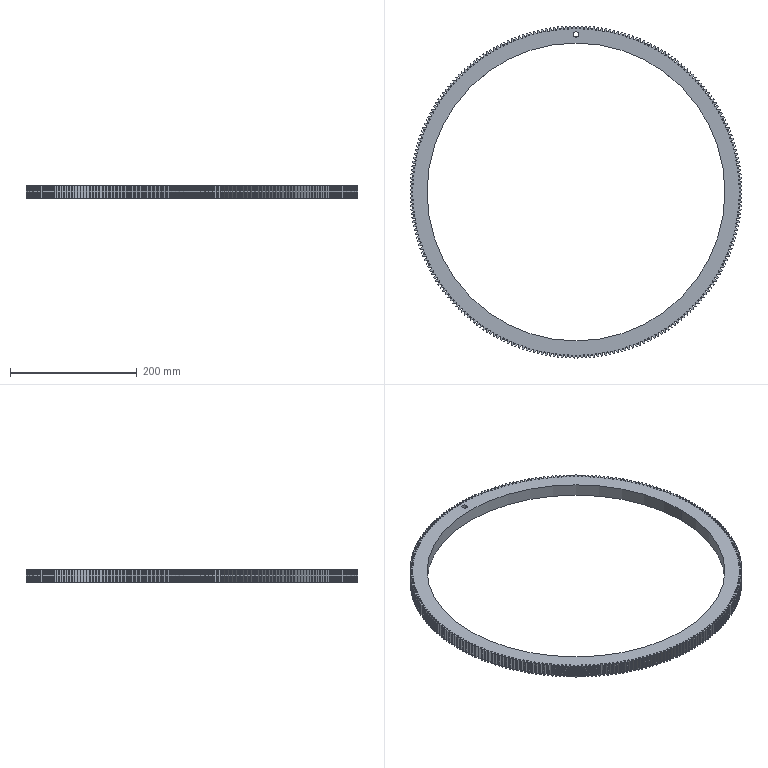Part | SolidWorks | features ICE 2, CirPattern 1, Extrusion 1, HoleWzd 1, RefAxis 1 | 1 solid | 1047 faces | box 523.979 x 523.979 x 20 mm | volume 771365 mm3 | cylinder 525 | spline 520 | plane 2 | commonest cylinder face diameters 514.994 x261 524 x260 8.5 x2 470 x2